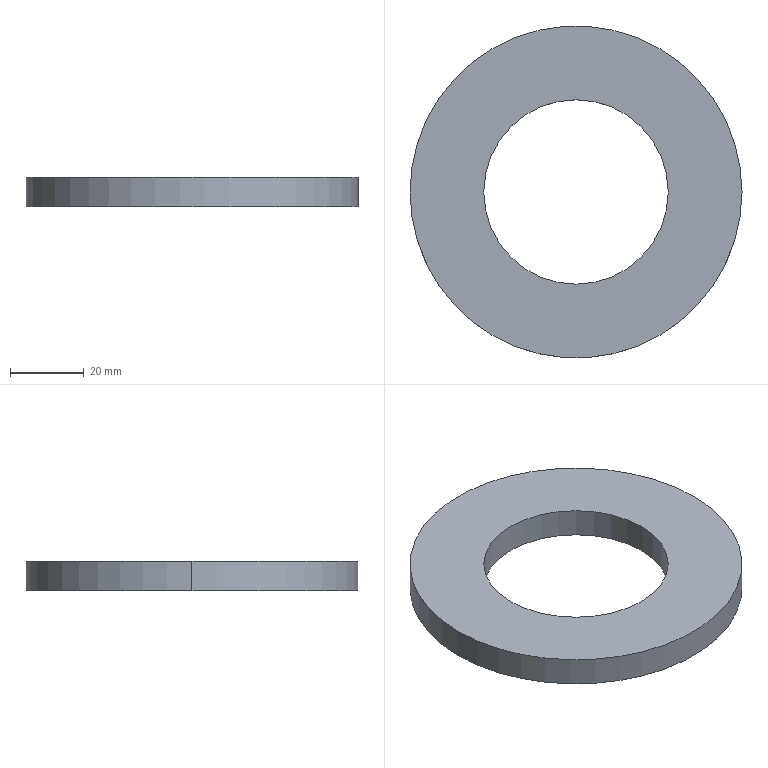Part | SolidWorks | features ICE 2, Chamfer 1, Cut 1, Extrusion 1 | 1 solid | 24 faces | box 90 x 90 x 8 mm | volume 34479 mm3 | cylinder 16 | plane 8 | commonest cylinder face diameters 5 x12 50 x2 90 x2
STEP:
#1=CARTESIAN_POINT('',(34.543,18.5,6.));
#2=VERTEX_POINT('',#1);
#3=CARTESIAN_POINT('',(29.543,18.5,6.));
#4=VERTEX_POINT('',#3);
#5=CARTESIAN_POINT('',(32.043,18.5,6.));
#6=DIRECTION('',(0.,0.,-1.));
#7=DIRECTION('',(-1.,0.,0.));
#8=AXIS2_PLACEMENT_3D('',#5,#6,#7);
#9=CIRCLE('',#8,2.5);
#10=EDGE_CURVE('',#2,#4,#9,.T.);
#11=ORIENTED_EDGE('',*,*,#10,.F.);
#12=CARTESIAN_POINT('',(34.543,18.5,0.));
#13=VERTEX_POINT('',#12);
#14=CARTESIAN_POINT('',(34.543,18.5,6.));
#15=DIRECTION('',(0.,0.,-1.));
#16=VECTOR('',#15,1000.);
#17=LINE('',#14,#16);
#18=EDGE_CURVE('',#2,#13,#17,.T.);
#19=ORIENTED_EDGE('',*,*,#18,.T.);
#20=CARTESIAN_POINT('',(29.543,18.5,0.));
#21=VERTEX_POINT('',#20);
#22=CARTESIAN_POINT('',(32.043,18.5,0.));
#23=DIRECTION('',(0.,0.,-1.));
#24=DIRECTION('',(-1.,0.,0.));
#25=AXIS2_PLACEMENT_3D('',#22,#23,#24);
#26=CIRCLE('',#25,2.5);
#27=EDGE_CURVE('',#13,#21,#26,.T.);
#28=ORIENTED_EDGE('',*,*,#27,.T.);
#29=CARTESIAN_POINT('',(29.543,18.5,6.));
#30=DIRECTION('',(0.,0.,-1.));
#31=VECTOR('',#30,1000.);
#32=LINE('',#29,#31);
#33=EDGE_CURVE('',#4,#21,#32,.T.);
#34=ORIENTED_EDGE('',*,*,#33,.F.);
#35=EDGE_LOOP('',(#11,#19,#28,#34));
#36=FACE_OUTER_BOUND('',#35,.T.);
#37=CARTESIAN_POINT('',(32.043,18.5,6.));
#38=DIRECTION('',(0.,0.,-1.));
#39=DIRECTION('',(-1.,0.,0.));
#40=AXIS2_PLACEMENT_3D('',#37,#38,#39);
#41=CYLINDRICAL_SURFACE('',#40,2.5);
#42=ADVANCED_FACE('',(#36),#41,.F.);
#43=CARTESIAN_POINT('',(34.543,-18.5,6.));
#44=VERTEX_POINT('',#43);
#45=CARTESIAN_POINT('',(29.543,-18.5,6.));
#46=VERTEX_POINT('',#45);
#47=CARTESIAN_POINT('',(32.043,-18.5,6.));
#48=DIRECTION('',(0.,0.,-1.));
#49=DIRECTION('',(-1.,0.,0.));
#50=AXIS2_PLACEMENT_3D('',#47,#48,#49);
#51=CIRCLE('',#50,2.5);
#52=EDGE_CURVE('',#44,#46,#51,.T.);
#53=ORIENTED_EDGE('',*,*,#52,.F.);
#54=CARTESIAN_POINT('',(34.543,-18.5,0.));
#55=VERTEX_POINT('',#54);
#56=CARTESIAN_POINT('',(34.543,-18.5,6.));
#57=DIRECTION('',(0.,0.,-1.));
#58=VECTOR('',#57,1000.);
#59=LINE('',#56,#58);
#60=EDGE_CURVE('',#44,#55,#59,.T.);
#61=ORIENTED_EDGE('',*,*,#60,.T.);
#62=CARTESIAN_POINT('',(29.543,-18.5,0.));
#63=VERTEX_POINT('',#62);
#64=CARTESIAN_POINT('',(32.043,-18.5,0.));
#65=DIRECTION('',(0.,0.,-1.));
#66=DIRECTION('',(-1.,0.,0.));
#67=AXIS2_PLACEMENT_3D('',#64,#65,#66);
#68=CIRCLE('',#67,2.5);
#69=EDGE_CURVE('',#55,#63,#68,.T.);
#70=ORIENTED_EDGE('',*,*,#69,.T.);
#71=CARTESIAN_POINT('',(29.543,-18.5,6.));
#72=DIRECTION('',(0.,0.,-1.));
#73=VECTOR('',#72,1000.);
#74=LINE('',#71,#73);
#75=EDGE_CURVE('',#46,#63,#74,.T.);
#76=ORIENTED_EDGE('',*,*,#75,.F.);
#77=EDGE_LOOP('',(#53,#61,#70,#76));
#78=FACE_OUTER_BOUND('',#77,.T.);
#79=CARTESIAN_POINT('',(32.043,-18.5,6.));
#80=DIRECTION('',(0.,0.,-1.));
#81=DIRECTION('',(-1.,0.,0.));
#82=AXIS2_PLACEMENT_3D('',#79,#80,#81);
#83=CYLINDRICAL_SURFACE('',#82,2.5);
#84=ADVANCED_FACE('',(#78),#83,.F.);
#85=CARTESIAN_POINT('',(2.5,-37.,6.));
#86=VERTEX_POINT('',#85);
#87=CARTESIAN_POINT('',(-2.5,-37.,6.));
#88=VERTEX_POINT('',#87);
#89=CARTESIAN_POINT('',(0.,-37.,6.));
#90=DIRECTION('',(0.,0.,-1.));
#91=DIRECTION('',(-1.,0.,0.));
#92=AXIS2_PLACEMENT_3D('',#89,#90,#91);
#93=CIRCLE('',#92,2.5);
#94=EDGE_CURVE('',#86,#88,#93,.T.);
#95=ORIENTED_EDGE('',*,*,#94,.F.);
#96=CARTESIAN_POINT('',(2.5,-37.,0.));
#97=VERTEX_POINT('',#96);
#98=CARTESIAN_POINT('',(2.5,-37.,6.));
#99=DIRECTION('',(0.,0.,-1.));
#100=VECTOR('',#99,1000.);
#101=LINE('',#98,#100);
#102=EDGE_CURVE('',#86,#97,#101,.T.);
#103=ORIENTED_EDGE('',*,*,#102,.T.);
#104=CARTESIAN_POINT('',(-2.5,-37.,0.));
#105=VERTEX_POINT('',#104);
#106=CARTESIAN_POINT('',(0.,-37.,0.));
#107=DIRECTION('',(0.,0.,-1.));
#108=DIRECTION('',(-1.,0.,0.));
#109=AXIS2_PLACEMENT_3D('',#106,#107,#108);
#110=CIRCLE('',#109,2.5);
#111=EDGE_CURVE('',#97,#105,#110,.T.);
#112=ORIENTED_EDGE('',*,*,#111,.T.);
#113=CARTESIAN_POINT('',(-2.5,-37.,6.));
#114=DIRECTION('',(0.,0.,-1.));
#115=VECTOR('',#114,1000.);
#116=LINE('',#113,#115);
#117=EDGE_CURVE('',#88,#105,#116,.T.);
#118=ORIENTED_EDGE('',*,*,#117,.F.);
#119=EDGE_LOOP('',(#95,#103,#112,#118));
#120=FACE_OUTER_BOUND('',#119,.T.);
#121=CARTESIAN_POINT('',(0.,-37.,6.));
#122=DIRECTION('',(0.,0.,-1.));
#123=DIRECTION('',(-1.,0.,0.));
#124=AXIS2_PLACEMENT_3D('',#121,#122,#123);
#125=CYLINDRICAL_SURFACE('',#124,2.5);
#126=ADVANCED_FACE('',(#120),#125,.F.);
#127=CARTESIAN_POINT('',(-29.543,-18.5,6.));
#128=VERTEX_POINT('',#127);
#129=CARTESIAN_POINT('',(-34.543,-18.5,6.));
#130=VERTEX_POINT('',#129);
#131=CARTESIAN_POINT('',(-32.043,-18.5,6.));
#132=DIRECTION('',(0.,0.,-1.));
#133=DIRECTION('',(-1.,0.,0.));
#134=AXIS2_PLACEMENT_3D('',#131,#132,#133);
#135=CIRCLE('',#134,2.5);
#136=EDGE_CURVE('',#128,#130,#135,.T.);
#137=ORIENTED_EDGE('',*,*,#136,.F.);
#138=CARTESIAN_POINT('',(-29.543,-18.5,0.));
#139=VERTEX_POINT('',#138);
#140=CARTESIAN_POINT('',(-29.543,-18.5,6.));
#141=DIRECTION('',(0.,0.,-1.));
#142=VECTOR('',#141,1000.);
#143=LINE('',#140,#142);
#144=EDGE_CURVE('',#128,#139,#143,.T.);
#145=ORIENTED_EDGE('',*,*,#144,.T.);
#146=CARTESIAN_POINT('',(-34.543,-18.5,0.));
#147=VERTEX_POINT('',#146);
#148=CARTESIAN_POINT('',(-32.043,-18.5,0.));
#149=DIRECTION('',(0.,0.,-1.));
#150=DIRECTION('',(-1.,0.,0.));
#151=AXIS2_PLACEMENT_3D('',#148,#149,#150);
#152=CIRCLE('',#151,2.5);
#153=EDGE_CURVE('',#139,#147,#152,.T.);
#154=ORIENTED_EDGE('',*,*,#153,.T.);
#155=CARTESIAN_POINT('',(-34.543,-18.5,6.));
#156=DIRECTION('',(0.,0.,-1.));
#157=VECTOR('',#156,1000.);
#158=LINE('',#155,#157);
#159=EDGE_CURVE('',#130,#147,#158,.T.);
#160=ORIENTED_EDGE('',*,*,#159,.F.);
#161=EDGE_LOOP('',(#137,#145,#154,#160));
#162=FACE_OUTER_BOUND('',#161,.T.);
#163=CARTESIAN_POINT('',(-32.043,-18.5,6.));
#164=DIRECTION('',(0.,0.,-1.));
#165=DIRECTION('',(-1.,0.,0.));
#166=AXIS2_PLACEMENT_3D('',#163,#164,#165);
#167=CYLINDRICAL_SURFACE('',#166,2.5);
#168=ADVANCED_FACE('',(#162),#167,.F.);
#169=CARTESIAN_POINT('',(-29.543,18.5,6.));
#170=VERTEX_POINT('',#169);
#171=CARTESIAN_POINT('',(-34.543,18.5,6.));
#172=VERTEX_POINT('',#171);
#173=CARTESIAN_POINT('',(-32.043,18.5,6.));
#174=DIRECTION('',(0.,0.,-1.));
#175=DIRECTION('',(-1.,0.,0.));
#176=AXIS2_PLACEMENT_3D('',#173,#174,#175);
#177=CIRCLE('',#176,2.5);
#178=EDGE_CURVE('',#170,#172,#177,.T.);
#179=ORIENTED_EDGE('',*,*,#178,.F.);
#180=CARTESIAN_POINT('',(-29.543,18.5,0.));
#181=VERTEX_POINT('',#180);
#182=CARTESIAN_POINT('',(-29.543,18.5,6.));
#183=DIRECTION('',(0.,0.,-1.));
#184=VECTOR('',#183,1000.);
#185=LINE('',#182,#184);
#186=EDGE_CURVE('',#170,#181,#185,.T.);
#187=ORIENTED_EDGE('',*,*,#186,.T.);
#188=CARTESIAN_POINT('',(-34.543,18.5,0.));
#189=VERTEX_POINT('',#188);
#190=CARTESIAN_POINT('',(-32.043,18.5,0.));
#191=DIRECTION('',(0.,0.,-1.));
#192=DIRECTION('',(-1.,0.,0.));
#193=AXIS2_PLACEMENT_3D('',#190,#191,#192);
#194=CIRCLE('',#193,2.5);
#195=EDGE_CURVE('',#181,#189,#194,.T.);
#196=ORIENTED_EDGE('',*,*,#195,.T.);
#197=CARTESIAN_POINT('',(-34.543,18.5,6.));
#198=DIRECTION('',(0.,0.,-1.));
#199=VECTOR('',#198,1000.);
#200=LINE('',#197,#199);
#201=EDGE_CURVE('',#172,#189,#200,.T.);
#202=ORIENTED_EDGE('',*,*,#201,.F.);
#203=EDGE_LOOP('',(#179,#187,#196,#202));
#204=FACE_OUTER_BOUND('',#203,.T.);
#205=CARTESIAN_POINT('',(-32.043,18.5,6.));
#206=DIRECTION('',(0.,0.,-1.));
#207=DIRECTION('',(-1.,0.,0.));
#208=AXIS2_PLACEMENT_3D('',#205,#206,#207);
#209=CYLINDRICAL_SURFACE('',#208,2.5);
#210=ADVANCED_FACE('',(#204),#209,.F.);
#211=CARTESIAN_POINT('',(2.5,37.,6.));
#212=VERTEX_POINT('',#211);
#213=CARTESIAN_POINT('',(-2.5,37.,6.));
#214=VERTEX_POINT('',#213);
#215=CARTESIAN_POINT('',(0.,37.,6.));
#216=DIRECTION('',(0.,0.,-1.));
#217=DIRECTION('',(-1.,0.,0.));
#218=AXIS2_PLACEMENT_3D('',#215,#216,#217);
#219=CIRCLE('',#218,2.5);
#220=EDGE_CURVE('',#212,#214,#219,.T.);
#221=ORIENTED_EDGE('',*,*,#220,.F.);
#222=CARTESIAN_POINT('',(2.5,37.,0.));
#223=VERTEX_POINT('',#222);
#224=CARTESIAN_POINT('',(2.5,37.,6.));
#225=DIRECTION('',(0.,0.,-1.));
#226=VECTOR('',#225,1000.);
#227=LINE('',#224,#226);
#228=EDGE_CURVE('',#212,#223,#227,.T.);
#229=ORIENTED_EDGE('',*,*,#228,.T.);
#230=CARTESIAN_POINT('',(-2.5,37.,0.));
#231=VERTEX_POINT('',#230);
#232=CARTESIAN_POINT('',(0.,37.,0.));
#233=DIRECTION('',(0.,0.,-1.));
#234=DIRECTION('',(-1.,0.,0.));
#235=AXIS2_PLACEMENT_3D('',#232,#233,#234);
#236=CIRCLE('',#235,2.5);
#237=EDGE_CURVE('',#223,#231,#236,.T.);
#238=ORIENTED_EDGE('',*,*,#237,.T.);
#239=CARTESIAN_POINT('',(-2.5,37.,6.));
#240=DIRECTION('',(0.,0.,-1.));
#241=VECTOR('',#240,1000.);
#242=LINE('',#239,#241);
#243=EDGE_CURVE('',#214,#231,#242,.T.);
#244=ORIENTED_EDGE('',*,*,#243,.F.);
#245=EDGE_LOOP('',(#221,#229,#238,#244));
#246=FACE_OUTER_BOUND('',#245,.T.);
#247=CARTESIAN_POINT('',(0.,37.,6.));
#248=DIRECTION('',(0.,0.,-1.));
#249=DIRECTION('',(-1.,0.,0.));
#250=AXIS2_PLACEMENT_3D('',#247,#248,#249);
#251=CYLINDRICAL_SURFACE('',#250,2.5);
#252=ADVANCED_FACE('',(#246),#251,.F.);
#253=CARTESIAN_POINT('',(25.,0.,8.));
#254=VERTEX_POINT('',#253);
#255=CARTESIAN_POINT('',(-25.,0.,8.));
#256=VERTEX_POINT('',#255);
#257=CARTESIAN_POINT('',(0.,0.,8.));
#258=DIRECTION('',(0.,0.,-1.));
#259=DIRECTION('',(-1.,0.,0.));
#260=AXIS2_PLACEMENT_3D('',#257,#258,#259);
#261=CIRCLE('',#260,25.);
#262=EDGE_CURVE('',#254,#256,#261,.T.);
#263=ORIENTED_EDGE('',*,*,#262,.F.);
#264=CARTESIAN_POINT('',(25.,0.,0.));
#265=VERTEX_POINT('',#264);
#266=CARTESIAN_POINT('',(25.,0.,8.));
#267=DIRECTION('',(0.,0.,-1.));
#268=VECTOR('',#267,1000.);
#269=LINE('',#266,#268);
#270=EDGE_CURVE('',#254,#265,#269,.T.);
#271=ORIENTED_EDGE('',*,*,#270,.T.);
#272=CARTESIAN_POINT('',(-25.,0.,0.));
#273=VERTEX_POINT('',#272);
#274=CARTESIAN_POINT('',(0.,0.,0.));
#275=DIRECTION('',(0.,0.,1.));
#276=DIRECTION('',(1.,0.,0.));
#277=AXIS2_PLACEMENT_3D('',#274,#275,#276);
#278=CIRCLE('',#277,25.);
#279=EDGE_CURVE('',#273,#265,#278,.T.);
#280=ORIENTED_EDGE('',*,*,#279,.F.);
#281=CARTESIAN_POINT('',(-25.,0.,8.));
#282=DIRECTION('',(0.,0.,-1.));
#283=VECTOR('',#282,1000.);
#284=LINE('',#281,#283);
#285=EDGE_CURVE('',#256,#273,#284,.T.);
#286=ORIENTED_EDGE('',*,*,#285,.F.);
#287=EDGE_LOOP('',(#263,#271,#280,#286));
#288=FACE_OUTER_BOUND('',#287,.T.);
#289=CARTESIAN_POINT('',(0.,0.,8.));
#290=DIRECTION('',(0.,0.,-1.));
#291=DIRECTION('',(-1.,0.,0.));
#292=AXIS2_PLACEMENT_3D('',#289,#290,#291);
#293=CYLINDRICAL_SURFACE('',#292,25.);
#294=ADVANCED_FACE('',(#288),#293,.F.);
#295=CARTESIAN_POINT('',(45.,0.,8.));
#296=VERTEX_POINT('',#295);
#297=CARTESIAN_POINT('',(-45.,0.,8.));
#298=VERTEX_POINT('',#297);
#299=CARTESIAN_POINT('',(0.,0.,8.));
#300=DIRECTION('',(0.,0.,1.));
#301=DIRECTION('',(1.,0.,0.));
#302=AXIS2_PLACEMENT_3D('',#299,#300,#301);
#303=CIRCLE('',#302,45.);
#304=EDGE_CURVE('',#296,#298,#303,.T.);
#305=ORIENTED_EDGE('',*,*,#304,.F.);
#306=CARTESIAN_POINT('',(45.,0.,0.));
#307=VERTEX_POINT('',#306);
#308=CARTESIAN_POINT('',(45.,0.,8.));
#309=DIRECTION('',(0.,0.,-1.));
#310=VECTOR('',#309,1000.);
#311=LINE('',#308,#310);
#312=EDGE_CURVE('',#296,#307,#311,.T.);
#313=ORIENTED_EDGE('',*,*,#312,.T.);
#314=CARTESIAN_POINT('',(-45.,0.,0.));
#315=VERTEX_POINT('',#314);
#316=CARTESIAN_POINT('',(0.,0.,0.));
#317=DIRECTION('',(0.,0.,1.));
#318=DIRECTION('',(1.,0.,0.));
#319=AXIS2_PLACEMENT_3D('',#316,#317,#318);
#320=CIRCLE('',#319,45.);
#321=EDGE_CURVE('',#307,#315,#320,.T.);
#322=ORIENTED_EDGE('',*,*,#321,.T.);
#323=CARTESIAN_POINT('',(-45.,0.,8.));
#324=DIRECTION('',(0.,0.,-1.));
#325=VECTOR('',#324,1000.);
#326=LINE('',#323,#325);
#327=EDGE_CURVE('',#298,#315,#326,.T.);
#328=ORIENTED_EDGE('',*,*,#327,.F.);
#329=EDGE_LOOP('',(#305,#313,#322,#328));
#330=FACE_OUTER_BOUND('',#329,.T.);
#331=CARTESIAN_POINT('',(0.,0.,8.));
#332=DIRECTION('',(0.,0.,-1.));
#333=DIRECTION('',(-1.,0.,0.));
#334=AXIS2_PLACEMENT_3D('',#331,#332,#333);
#335=CYLINDRICAL_SURFACE('',#334,45.);
#336=ADVANCED_FACE('',(#330),#335,.T.);
#337=CARTESIAN_POINT('',(0.,0.,8.));
#338=DIRECTION('',(0.,0.,1.));
#339=DIRECTION('',(1.,0.,0.));
#340=AXIS2_PLACEMENT_3D('',#337,#338,#339);
#341=CIRCLE('',#340,45.);
#342=EDGE_CURVE('',#298,#296,#341,.T.);
#343=ORIENTED_EDGE('',*,*,#342,.T.);
#344=ORIENTED_EDGE('',*,*,#304,.T.);
#345=EDGE_LOOP('',(#343,#344));
#346=FACE_OUTER_BOUND('',#345,.T.);
#347=CARTESIAN_POINT('',(0.,0.,8.));
#348=DIRECTION('',(0.,0.,-1.));
#349=DIRECTION('',(-1.,0.,0.));
#350=AXIS2_PLACEMENT_3D('',#347,#348,#349);
#351=CIRCLE('',#350,25.);
#352=EDGE_CURVE('',#256,#254,#351,.T.);
#353=ORIENTED_EDGE('',*,*,#352,.T.);
#354=ORIENTED_EDGE('',*,*,#262,.T.);
#355=EDGE_LOOP('',(#353,#354));
#356=FACE_BOUND('',#355,.T.);
#357=CARTESIAN_POINT('',(0.,0.,8.));
#358=DIRECTION('',(0.,0.,1.));
#359=DIRECTION('',(1.,0.,0.));
#360=AXIS2_PLACEMENT_3D('',#357,#358,#359);
#361=PLANE('',#360);
#362=ADVANCED_FACE('',(#346,#356),#361,.T.);
#363=CARTESIAN_POINT('',(32.043,18.5,0.));
#364=DIRECTION('',(0.,0.,-1.));
#365=DIRECTION('',(-1.,0.,0.));
#366=AXIS2_PLACEMENT_3D('',#363,#364,#365);
#367=CIRCLE('',#366,2.5);
#368=EDGE_CURVE('',#21,#13,#367,.T.);
#369=ORIENTED_EDGE('',*,*,#368,.F.);
#370=ORIENTED_EDGE('',*,*,#27,.F.);
#371=EDGE_LOOP('',(#369,#370));
#372=FACE_BOUND('',#371,.T.);
#373=CARTESIAN_POINT('',(32.043,-18.5,0.));
#374=DIRECTION('',(0.,0.,-1.));
#375=DIRECTION('',(-1.,0.,0.));
#376=AXIS2_PLACEMENT_3D('',#373,#374,#375);
#377=CIRCLE('',#376,2.5);
#378=EDGE_CURVE('',#63,#55,#377,.T.);
#379=ORIENTED_EDGE('',*,*,#378,.F.);
#380=ORIENTED_EDGE('',*,*,#69,.F.);
#381=EDGE_LOOP('',(#379,#380));
#382=FACE_BOUND('',#381,.T.);
#383=CARTESIAN_POINT('',(0.,-37.,0.));
#384=DIRECTION('',(0.,0.,-1.));
#385=DIRECTION('',(-1.,0.,0.));
#386=AXIS2_PLACEMENT_3D('',#383,#384,#385);
#387=CIRCLE('',#386,2.5);
#388=EDGE_CURVE('',#105,#97,#387,.T.);
#389=ORIENTED_EDGE('',*,*,#388,.F.);
#390=ORIENTED_EDGE('',*,*,#111,.F.);
#391=EDGE_LOOP('',(#389,#390));
#392=FACE_BOUND('',#391,.T.);
#393=CARTESIAN_POINT('',(-32.043,-18.5,0.));
#394=DIRECTION('',(0.,0.,-1.));
#395=DIRECTION('',(-1.,0.,0.));
#396=AXIS2_PLACEMENT_3D('',#393,#394,#395);
#397=CIRCLE('',#396,2.5);
#398=EDGE_CURVE('',#147,#139,#397,.T.);
#399=ORIENTED_EDGE('',*,*,#398,.F.);
#400=ORIENTED_EDGE('',*,*,#153,.F.);
#401=EDGE_LOOP('',(#399,#400));
#402=FACE_BOUND('',#401,.T.);
#403=CARTESIAN_POINT('',(-32.043,18.5,0.));
#404=DIRECTION('',(0.,0.,-1.));
#405=DIRECTION('',(-1.,0.,0.));
#406=AXIS2_PLACEMENT_3D('',#403,#404,#405);
#407=CIRCLE('',#406,2.5);
#408=EDGE_CURVE('',#189,#181,#407,.T.);
#409=ORIENTED_EDGE('',*,*,#408,.F.);
#410=ORIENTED_EDGE('',*,*,#195,.F.);
#411=EDGE_LOOP('',(#409,#410));
#412=FACE_BOUND('',#411,.T.);
#413=CARTESIAN_POINT('',(0.,37.,0.));
#414=DIRECTION('',(0.,0.,-1.));
#415=DIRECTION('',(-1.,0.,0.));
#416=AXIS2_PLACEMENT_3D('',#413,#414,#415);
#417=CIRCLE('',#416,2.5);
#418=EDGE_CURVE('',#231,#223,#417,.T.);
#419=ORIENTED_EDGE('',*,*,#418,.F.);
#420=ORIENTED_EDGE('',*,*,#237,.F.);
#421=EDGE_LOOP('',(#419,#420));
#422=FACE_BOUND('',#421,.T.);
#423=CARTESIAN_POINT('',(0.,0.,0.));
#424=DIRECTION('',(0.,0.,1.));
#425=DIRECTION('',(1.,0.,0.));
#426=AXIS2_PLACEMENT_3D('',#423,#424,#425);
#427=CIRCLE('',#426,45.);
#428=EDGE_CURVE('',#315,#307,#427,.T.);
#429=ORIENTED_EDGE('',*,*,#428,.F.);
#430=ORIENTED_EDGE('',*,*,#321,.F.);
#431=EDGE_LOOP('',(#429,#430));
#432=FACE_OUTER_BOUND('',#431,.T.);
#433=ORIENTED_EDGE('',*,*,#279,.T.);
#434=CARTESIAN_POINT('',(0.,0.,0.));
#435=DIRECTION('',(0.,0.,1.));
#436=DIRECTION('',(1.,0.,0.));
#437=AXIS2_PLACEMENT_3D('',#434,#435,#436);
#438=CIRCLE('',#437,25.);
#439=EDGE_CURVE('',#265,#273,#438,.T.);
#440=ORIENTED_EDGE('',*,*,#439,.T.);
#441=EDGE_LOOP('',(#433,#440));
#442=FACE_BOUND('',#441,.T.);
#443=CARTESIAN_POINT('',(0.,0.,0.));
#444=DIRECTION('',(0.,0.,1.));
#445=DIRECTION('',(1.,0.,0.));
#446=AXIS2_PLACEMENT_3D('',#443,#444,#445);
#447=PLANE('',#446);
#448=ADVANCED_FACE('',(#372,#382,#392,#402,#412,#422,#432,#442),#447,.F.);
#449=ORIENTED_EDGE('',*,*,#312,.F.);
#450=ORIENTED_EDGE('',*,*,#342,.F.);
#451=ORIENTED_EDGE('',*,*,#327,.T.);
#452=ORIENTED_EDGE('',*,*,#428,.T.);
#453=EDGE_LOOP('',(#449,#450,#451,#452));
#454=FACE_OUTER_BOUND('',#453,.T.);
#455=CARTESIAN_POINT('',(0.,0.,8.));
#456=DIRECTION('',(0.,0.,-1.));
#457=DIRECTION('',(-1.,0.,0.));
#458=AXIS2_PLACEMENT_3D('',#455,#456,#457);
#459=CYLINDRICAL_SURFACE('',#458,45.);
#460=ADVANCED_FACE('',(#454),#459,.T.);
#461=ORIENTED_EDGE('',*,*,#270,.F.);
#462=ORIENTED_EDGE('',*,*,#352,.F.);
#463=ORIENTED_EDGE('',*,*,#285,.T.);
#464=ORIENTED_EDGE('',*,*,#439,.F.);
#465=EDGE_LOOP('',(#461,#462,#463,#464));
#466=FACE_OUTER_BOUND('',#465,.T.);
#467=CARTESIAN_POINT('',(0.,0.,8.));
#468=DIRECTION('',(0.,0.,-1.));
#469=DIRECTION('',(-1.,0.,0.));
#470=AXIS2_PLACEMENT_3D('',#467,#468,#469);
#471=CYLINDRICAL_SURFACE('',#470,25.);
#472=ADVANCED_FACE('',(#466),#471,.F.);
#473=ORIENTED_EDGE('',*,*,#228,.F.);
#474=CARTESIAN_POINT('',(0.,37.,6.));
#475=DIRECTION('',(0.,0.,-1.));
#476=DIRECTION('',(-1.,0.,0.));
#477=AXIS2_PLACEMENT_3D('',#474,#475,#476);
#478=CIRCLE('',#477,2.5);
#479=EDGE_CURVE('',#214,#212,#478,.T.);
#480=ORIENTED_EDGE('',*,*,#479,.F.);
#481=ORIENTED_EDGE('',*,*,#243,.T.);
#482=ORIENTED_EDGE('',*,*,#418,.T.);
#483=EDGE_LOOP('',(#473,#480,#481,#482));
#484=FACE_OUTER_BOUND('',#483,.T.);
#485=CARTESIAN_POINT('',(0.,37.,6.));
#486=DIRECTION('',(0.,0.,-1.));
#487=DIRECTION('',(-1.,0.,0.));
#488=AXIS2_PLACEMENT_3D('',#485,#486,#487);
#489=CYLINDRICAL_SURFACE('',#488,2.5);
#490=ADVANCED_FACE('',(#484),#489,.F.);
#491=ORIENTED_EDGE('',*,*,#479,.T.);
#492=ORIENTED_EDGE('',*,*,#220,.T.);
#493=EDGE_LOOP('',(#491,#492));
#494=FACE_OUTER_BOUND('',#493,.T.);
#495=CARTESIAN_POINT('',(0.,37.,6.));
#496=DIRECTION('',(0.,0.,-1.));
#497=DIRECTION('',(-1.,0.,0.));
#498=AXIS2_PLACEMENT_3D('',#495,#496,#497);
#499=PLANE('',#498);
#500=ADVANCED_FACE('',(#494),#499,.T.);
#501=ORIENTED_EDGE('',*,*,#186,.F.);
#502=CARTESIAN_POINT('',(-32.043,18.5,6.));
#503=DIRECTION('',(0.,0.,-1.));
#504=DIRECTION('',(-1.,0.,0.));
#505=AXIS2_PLACEMENT_3D('',#502,#503,#504);
#506=CIRCLE('',#505,2.5);
#507=EDGE_CURVE('',#172,#170,#506,.T.);
#508=ORIENTED_EDGE('',*,*,#507,.F.);
#509=ORIENTED_EDGE('',*,*,#201,.T.);
#510=ORIENTED_EDGE('',*,*,#408,.T.);
#511=EDGE_LOOP('',(#501,#508,#509,#510));
#512=FACE_OUTER_BOUND('',#511,.T.);
#513=CARTESIAN_POINT('',(-32.043,18.5,6.));
#514=DIRECTION('',(0.,0.,-1.));
#515=DIRECTION('',(-1.,0.,0.));
#516=AXIS2_PLACEMENT_3D('',#513,#514,#515);
#517=CYLINDRICAL_SURFACE('',#516,2.5);
#518=ADVANCED_FACE('',(#512),#517,.F.);
#519=ORIENTED_EDGE('',*,*,#507,.T.);
#520=ORIENTED_EDGE('',*,*,#178,.T.);
#521=EDGE_LOOP('',(#519,#520));
#522=FACE_OUTER_BOUND('',#521,.T.);
#523=CARTESIAN_POINT('',(-32.043,18.5,6.));
#524=DIRECTION('',(0.,0.,-1.));
#525=DIRECTION('',(-1.,0.,0.));
#526=AXIS2_PLACEMENT_3D('',#523,#524,#525);
#527=PLANE('',#526);
#528=ADVANCED_FACE('',(#522),#527,.T.);
#529=ORIENTED_EDGE('',*,*,#144,.F.);
#530=CARTESIAN_POINT('',(-32.043,-18.5,6.));
#531=DIRECTION('',(0.,0.,-1.));
#532=DIRECTION('',(-1.,0.,0.));
#533=AXIS2_PLACEMENT_3D('',#530,#531,#532);
#534=CIRCLE('',#533,2.5);
#535=EDGE_CURVE('',#130,#128,#534,.T.);
#536=ORIENTED_EDGE('',*,*,#535,.F.);
#537=ORIENTED_EDGE('',*,*,#159,.T.);
#538=ORIENTED_EDGE('',*,*,#398,.T.);
#539=EDGE_LOOP('',(#529,#536,#537,#538));
#540=FACE_OUTER_BOUND('',#539,.T.);
#541=CARTESIAN_POINT('',(-32.043,-18.5,6.));
#542=DIRECTION('',(0.,0.,-1.));
#543=DIRECTION('',(-1.,0.,0.));
#544=AXIS2_PLACEMENT_3D('',#541,#542,#543);
#545=CYLINDRICAL_SURFACE('',#544,2.5);
#546=ADVANCED_FACE('',(#540),#545,.F.);
#547=ORIENTED_EDGE('',*,*,#535,.T.);
#548=ORIENTED_EDGE('',*,*,#136,.T.);
#549=EDGE_LOOP('',(#547,#548));
#550=FACE_OUTER_BOUND('',#549,.T.);
#551=CARTESIAN_POINT('',(-32.043,-18.5,6.));
#552=DIRECTION('',(0.,0.,-1.));
#553=DIRECTION('',(-1.,0.,0.));
#554=AXIS2_PLACEMENT_3D('',#551,#552,#553);
#555=PLANE('',#554);
#556=ADVANCED_FACE('',(#550),#555,.T.);
#557=ORIENTED_EDGE('',*,*,#102,.F.);
#558=CARTESIAN_POINT('',(0.,-37.,6.));
#559=DIRECTION('',(0.,0.,-1.));
#560=DIRECTION('',(-1.,0.,0.));
#561=AXIS2_PLACEMENT_3D('',#558,#559,#560);
#562=CIRCLE('',#561,2.5);
#563=EDGE_CURVE('',#88,#86,#562,.T.);
#564=ORIENTED_EDGE('',*,*,#563,.F.);
#565=ORIENTED_EDGE('',*,*,#117,.T.);
#566=ORIENTED_EDGE('',*,*,#388,.T.);
#567=EDGE_LOOP('',(#557,#564,#565,#566));
#568=FACE_OUTER_BOUND('',#567,.T.);
#569=CARTESIAN_POINT('',(0.,-37.,6.));
#570=DIRECTION('',(0.,0.,-1.));
#571=DIRECTION('',(-1.,0.,0.));
#572=AXIS2_PLACEMENT_3D('',#569,#570,#571);
#573=CYLINDRICAL_SURFACE('',#572,2.5);
#574=ADVANCED_FACE('',(#568),#573,.F.);
#575=ORIENTED_EDGE('',*,*,#563,.T.);
#576=ORIENTED_EDGE('',*,*,#94,.T.);
#577=EDGE_LOOP('',(#575,#576));
#578=FACE_OUTER_BOUND('',#577,.T.);
#579=CARTESIAN_POINT('',(0.,-37.,6.));
#580=DIRECTION('',(0.,0.,-1.));
#581=DIRECTION('',(-1.,0.,0.));
#582=AXIS2_PLACEMENT_3D('',#579,#580,#581);
#583=PLANE('',#582);
#584=ADVANCED_FACE('',(#578),#583,.T.);
#585=ORIENTED_EDGE('',*,*,#60,.F.);
#586=CARTESIAN_POINT('',(32.043,-18.5,6.));
#587=DIRECTION('',(0.,0.,-1.));
#588=DIRECTION('',(-1.,0.,0.));
#589=AXIS2_PLACEMENT_3D('',#586,#587,#588);
#590=CIRCLE('',#589,2.5);
#591=EDGE_CURVE('',#46,#44,#590,.T.);
#592=ORIENTED_EDGE('',*,*,#591,.F.);
#593=ORIENTED_EDGE('',*,*,#75,.T.);
#594=ORIENTED_EDGE('',*,*,#378,.T.);
#595=EDGE_LOOP('',(#585,#592,#593,#594));
#596=FACE_OUTER_BOUND('',#595,.T.);
#597=CARTESIAN_POINT('',(32.043,-18.5,6.));
#598=DIRECTION('',(0.,0.,-1.));
#599=DIRECTION('',(-1.,0.,0.));
#600=AXIS2_PLACEMENT_3D('',#597,#598,#599);
#601=CYLINDRICAL_SURFACE('',#600,2.5);
#602=ADVANCED_FACE('',(#596),#601,.F.);
#603=ORIENTED_EDGE('',*,*,#591,.T.);
#604=ORIENTED_EDGE('',*,*,#52,.T.);
#605=EDGE_LOOP('',(#603,#604));
#606=FACE_OUTER_BOUND('',#605,.T.);
#607=CARTESIAN_POINT('',(32.043,-18.5,6.));
#608=DIRECTION('',(0.,0.,-1.));
#609=DIRECTION('',(-1.,0.,0.));
#610=AXIS2_PLACEMENT_3D('',#607,#608,#609);
#611=PLANE('',#610);
#612=ADVANCED_FACE('',(#606),#611,.T.);
#613=ORIENTED_EDGE('',*,*,#18,.F.);
#614=CARTESIAN_POINT('',(32.043,18.5,6.));
#615=DIRECTION('',(0.,0.,-1.));
#616=DIRECTION('',(-1.,0.,0.));
#617=AXIS2_PLACEMENT_3D('',#614,#615,#616);
#618=CIRCLE('',#617,2.5);
#619=EDGE_CURVE('',#4,#2,#618,.T.);
#620=ORIENTED_EDGE('',*,*,#619,.F.);
#621=ORIENTED_EDGE('',*,*,#33,.T.);
#622=ORIENTED_EDGE('',*,*,#368,.T.);
#623=EDGE_LOOP('',(#613,#620,#621,#622));
#624=FACE_OUTER_BOUND('',#623,.T.);
#625=CARTESIAN_POINT('',(32.043,18.5,6.));
#626=DIRECTION('',(0.,0.,-1.));
#627=DIRECTION('',(-1.,0.,0.));
#628=AXIS2_PLACEMENT_3D('',#625,#626,#627);
#629=CYLINDRICAL_SURFACE('',#628,2.5);
#630=ADVANCED_FACE('',(#624),#629,.F.);
#631=ORIENTED_EDGE('',*,*,#619,.T.);
#632=ORIENTED_EDGE('',*,*,#10,.T.);
#633=EDGE_LOOP('',(#631,#632));
#634=FACE_OUTER_BOUND('',#633,.T.);
#635=CARTESIAN_POINT('',(32.043,18.5,6.));
#636=DIRECTION('',(0.,0.,-1.));
#637=DIRECTION('',(-1.,0.,0.));
#638=AXIS2_PLACEMENT_3D('',#635,#636,#637);
#639=PLANE('',#638);
#640=ADVANCED_FACE('',(#634),#639,.T.);
#641=CLOSED_SHELL('',(#42,#84,#126,#168,#210,#252,#294,#336,#362,#448,#460,#472,#490,#500,#518,#528,#546,#556,#574,#584,#602,#612,#630,#640));
#642=MANIFOLD_SOLID_BREP('',#641);
#643=CARTESIAN_POINT('',(0.,0.,0.));
#644=DIRECTION('',(0.,0.,1.));
#645=DIRECTION('',(1.,0.,0.));
#646=AXIS2_PLACEMENT_3D('',#643,#644,#645);
#647=(LENGTH_UNIT()NAMED_UNIT(*)SI_UNIT(.MILLI.,.METRE.));
#648=UNCERTAINTY_MEASURE_WITH_UNIT(LENGTH_MEASURE(0.00001),#647,'','');
#649=(NAMED_UNIT(*)PLANE_ANGLE_UNIT()SI_UNIT($,.RADIAN.));
#650=(NAMED_UNIT(*)SI_UNIT($,.STERADIAN.)SOLID_ANGLE_UNIT());
#651=(GEOMETRIC_REPRESENTATION_CONTEXT(3)GLOBAL_UNCERTAINTY_ASSIGNED_CONTEXT((#648))GLOBAL_UNIT_ASSIGNED_CONTEXT((#647,#649,#650))REPRESENTATION_CONTEXT('',''));
#652=ADVANCED_BREP_SHAPE_REPRESENTATION('',(#642,#646),#651);